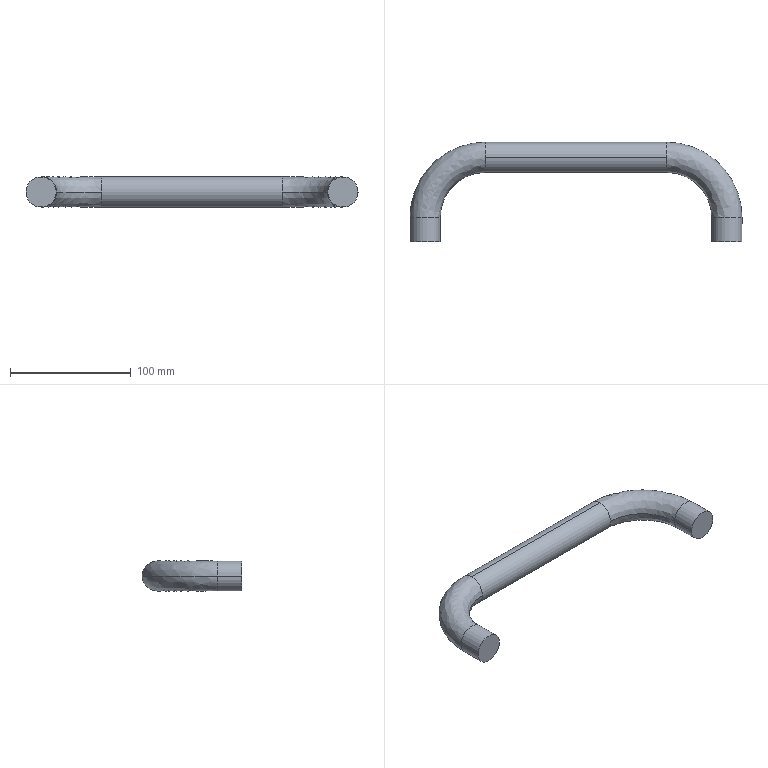Part | STEP file | 750078419 | 1 solid | 12 faces | box 275 x 82.5 x 25 mm | volume 170372 mm3 | cylinder 6 | spline 4 | plane 2 | commonest cylinder face diameters 25 x6
STEP:
#1=CARTESIAN_POINT('',(200.,82.5,0.));
#2=VERTEX_POINT('',#1);
#3=CARTESIAN_POINT('',(200.,70.,-12.5));
#4=VERTEX_POINT('',#3);
#5=CARTESIAN_POINT('',(200.,70.,0.));
#6=DIRECTION('',(-1.,0.,0.));
#7=DIRECTION('',(0.,0.,1.));
#8=AXIS2_PLACEMENT_3D('',#5,#6,#7);
#9=CIRCLE('',#8,12.5);
#10=EDGE_CURVE('',#2,#4,#9,.T.);
#11=ORIENTED_EDGE('',*,*,#10,.T.);
#12=CARTESIAN_POINT('',(50.,70.,-12.5));
#13=VERTEX_POINT('',#12);
#14=CARTESIAN_POINT('',(200.,70.,-12.5));
#15=DIRECTION('',(-1.,0.,0.));
#16=VECTOR('',#15,1000.);
#17=LINE('',#14,#16);
#18=EDGE_CURVE('',#4,#13,#17,.T.);
#19=ORIENTED_EDGE('',*,*,#18,.T.);
#20=CARTESIAN_POINT('',(50.,82.5,0.));
#21=VERTEX_POINT('',#20);
#22=CARTESIAN_POINT('',(50.,70.,0.));
#23=DIRECTION('',(1.,0.,0.));
#24=DIRECTION('',(0.,0.,1.));
#25=AXIS2_PLACEMENT_3D('',#22,#23,#24);
#26=CIRCLE('',#25,12.5);
#27=EDGE_CURVE('',#13,#21,#26,.T.);
#28=ORIENTED_EDGE('',*,*,#27,.T.);
#29=CARTESIAN_POINT('',(50.,70.,12.5));
#30=VERTEX_POINT('',#29);
#31=CARTESIAN_POINT('',(50.,70.,0.));
#32=DIRECTION('',(1.,0.,0.));
#33=DIRECTION('',(0.,0.,1.));
#34=AXIS2_PLACEMENT_3D('',#31,#32,#33);
#35=CIRCLE('',#34,12.5);
#36=EDGE_CURVE('',#21,#30,#35,.T.);
#37=ORIENTED_EDGE('',*,*,#36,.T.);
#38=CARTESIAN_POINT('',(200.,70.,12.5));
#39=VERTEX_POINT('',#38);
#40=CARTESIAN_POINT('',(200.,70.,12.5));
#41=DIRECTION('',(-1.,0.,0.));
#42=VECTOR('',#41,1000.);
#43=LINE('',#40,#42);
#44=EDGE_CURVE('',#39,#30,#43,.T.);
#45=ORIENTED_EDGE('',*,*,#44,.F.);
#46=CARTESIAN_POINT('',(200.,70.,0.));
#47=DIRECTION('',(-1.,0.,0.));
#48=DIRECTION('',(0.,0.,1.));
#49=AXIS2_PLACEMENT_3D('',#46,#47,#48);
#50=CIRCLE('',#49,12.5);
#51=EDGE_CURVE('',#39,#2,#50,.T.);
#52=ORIENTED_EDGE('',*,*,#51,.T.);
#53=EDGE_LOOP('',(#11,#19,#28,#37,#45,#52));
#54=FACE_OUTER_BOUND('',#53,.T.);
#55=CARTESIAN_POINT('',(200.,70.,0.));
#56=DIRECTION('',(-1.,0.,0.));
#57=DIRECTION('',(0.,0.,1.));
#58=AXIS2_PLACEMENT_3D('',#55,#56,#57);
#59=CYLINDRICAL_SURFACE('',#58,12.5);
#60=ADVANCED_FACE('',(#54),#59,.T.);
#61=CARTESIAN_POINT('',(50.,57.5,0.));
#62=VERTEX_POINT('',#61);
#63=CARTESIAN_POINT('',(50.,70.,0.));
#64=DIRECTION('',(1.,0.,0.));
#65=DIRECTION('',(0.,0.,1.));
#66=AXIS2_PLACEMENT_3D('',#63,#64,#65);
#67=CIRCLE('',#66,12.5);
#68=EDGE_CURVE('',#62,#13,#67,.T.);
#69=ORIENTED_EDGE('',*,*,#68,.F.);
#70=CARTESIAN_POINT('',(12.5,20.,0.));
#71=VERTEX_POINT('',#70);
#72=CARTESIAN_POINT('',(50.,20.,0.));
#73=DIRECTION('',(0.,0.,1.));
#74=DIRECTION('',(1.,0.,0.));
#75=AXIS2_PLACEMENT_3D('',#72,#73,#74);
#76=CIRCLE('',#75,37.5);
#77=EDGE_CURVE('',#62,#71,#76,.T.);
#78=ORIENTED_EDGE('',*,*,#77,.T.);
#79=CARTESIAN_POINT('',(-12.5,20.,0.));
#80=VERTEX_POINT('',#79);
#81=CARTESIAN_POINT('',(0.,20.,0.));
#82=DIRECTION('',(0.,1.,0.));
#83=DIRECTION('',(-1.,0.,0.));
#84=AXIS2_PLACEMENT_3D('',#81,#82,#83);
#85=CIRCLE('',#84,12.5);
#86=EDGE_CURVE('',#71,#80,#85,.T.);
#87=ORIENTED_EDGE('',*,*,#86,.T.);
#88=CARTESIAN_POINT('',(50.,20.,0.));
#89=DIRECTION('',(0.,0.,1.));
#90=DIRECTION('',(1.,0.,0.));
#91=AXIS2_PLACEMENT_3D('',#88,#89,#90);
#92=CIRCLE('',#91,62.5);
#93=EDGE_CURVE('',#21,#80,#92,.T.);
#94=ORIENTED_EDGE('',*,*,#93,.F.);
#95=ORIENTED_EDGE('',*,*,#27,.F.);
#96=EDGE_LOOP('',(#69,#78,#87,#94,#95));
#97=FACE_OUTER_BOUND('',#96,.T.);
#98=CARTESIAN_POINT('',(50.,82.5,0.));
#99=CARTESIAN_POINT('',(13.388,82.5,0.));
#100=CARTESIAN_POINT('',(-12.5,56.612,0.));
#101=CARTESIAN_POINT('',(-12.5,20.,0.));
#102=CARTESIAN_POINT('',(50.,82.5,-25.));
#103=CARTESIAN_POINT('',(13.388,82.5,-25.));
#104=CARTESIAN_POINT('',(-12.5,56.612,-25.));
#105=CARTESIAN_POINT('',(-12.5,20.,-25.));
#106=CARTESIAN_POINT('',(50.,57.5,-25.));
#107=CARTESIAN_POINT('',(28.033,57.5,-25.));
#108=CARTESIAN_POINT('',(12.5,41.967,-25.));
#109=CARTESIAN_POINT('',(12.5,20.,-25.));
#110=CARTESIAN_POINT('',(50.,57.5,0.));
#111=CARTESIAN_POINT('',(28.033,57.5,0.));
#112=CARTESIAN_POINT('',(12.5,41.967,0.));
#113=CARTESIAN_POINT('',(12.5,20.,0.));
#114=(BOUNDED_SURFACE()B_SPLINE_SURFACE(3,3,((#98,#99,#100,#101),(#102,#103,#104,#105),(#106,#107,#108,#109),(#110,#111,#112,#113)),.UNSPECIFIED.,.F.,.F.,.F.)B_SPLINE_SURFACE_WITH_KNOTS((4,4),(4,4),(0.,1.),(0.,1.),.UNSPECIFIED.)GEOMETRIC_REPRESENTATION_ITEM()RATIONAL_B_SPLINE_SURFACE(((1.,0.8047,0.8047,1.),(0.3333,0.2682,0.2682,0.3333),(0.3333,0.2682,0.2682,0.3333),(1.,0.8047,0.8047,1.)))REPRESENTATION_ITEM('')SURFACE());
#115=ADVANCED_FACE('',(#97),#114,.T.);
#116=CARTESIAN_POINT('',(262.5,20.,0.));
#117=VERTEX_POINT('',#116);
#118=CARTESIAN_POINT('',(237.5,20.,0.));
#119=VERTEX_POINT('',#118);
#120=CARTESIAN_POINT('',(250.,20.,0.));
#121=DIRECTION('',(0.,1.,0.));
#122=DIRECTION('',(1.,0.,0.));
#123=AXIS2_PLACEMENT_3D('',#120,#121,#122);
#124=CIRCLE('',#123,12.5);
#125=EDGE_CURVE('',#117,#119,#124,.T.);
#126=ORIENTED_EDGE('',*,*,#125,.T.);
#127=CARTESIAN_POINT('',(200.,57.5,0.));
#128=VERTEX_POINT('',#127);
#129=CARTESIAN_POINT('',(200.,20.,0.));
#130=DIRECTION('',(0.,0.,1.));
#131=DIRECTION('',(1.,0.,0.));
#132=AXIS2_PLACEMENT_3D('',#129,#130,#131);
#133=CIRCLE('',#132,37.5);
#134=EDGE_CURVE('',#119,#128,#133,.T.);
#135=ORIENTED_EDGE('',*,*,#134,.T.);
#136=CARTESIAN_POINT('',(200.,70.,0.));
#137=DIRECTION('',(-1.,0.,0.));
#138=DIRECTION('',(0.,0.,1.));
#139=AXIS2_PLACEMENT_3D('',#136,#137,#138);
#140=CIRCLE('',#139,12.5);
#141=EDGE_CURVE('',#4,#128,#140,.T.);
#142=ORIENTED_EDGE('',*,*,#141,.F.);
#143=ORIENTED_EDGE('',*,*,#10,.F.);
#144=CARTESIAN_POINT('',(200.,20.,0.));
#145=DIRECTION('',(0.,0.,1.));
#146=DIRECTION('',(1.,0.,0.));
#147=AXIS2_PLACEMENT_3D('',#144,#145,#146);
#148=CIRCLE('',#147,62.5);
#149=EDGE_CURVE('',#117,#2,#148,.T.);
#150=ORIENTED_EDGE('',*,*,#149,.F.);
#151=EDGE_LOOP('',(#126,#135,#142,#143,#150));
#152=FACE_OUTER_BOUND('',#151,.T.);
#153=CARTESIAN_POINT('',(262.5,20.,0.));
#154=CARTESIAN_POINT('',(262.5,56.612,0.));
#155=CARTESIAN_POINT('',(236.612,82.5,0.));
#156=CARTESIAN_POINT('',(200.,82.5,0.));
#157=CARTESIAN_POINT('',(262.5,20.,-25.));
#158=CARTESIAN_POINT('',(262.5,56.612,-25.));
#159=CARTESIAN_POINT('',(236.612,82.5,-25.));
#160=CARTESIAN_POINT('',(200.,82.5,-25.));
#161=CARTESIAN_POINT('',(237.5,20.,-25.));
#162=CARTESIAN_POINT('',(237.5,41.967,-25.));
#163=CARTESIAN_POINT('',(221.967,57.5,-25.));
#164=CARTESIAN_POINT('',(200.,57.5,-25.));
#165=CARTESIAN_POINT('',(237.5,20.,0.));
#166=CARTESIAN_POINT('',(237.5,41.967,0.));
#167=CARTESIAN_POINT('',(221.967,57.5,0.));
#168=CARTESIAN_POINT('',(200.,57.5,0.));
#169=(BOUNDED_SURFACE()B_SPLINE_SURFACE(3,3,((#153,#154,#155,#156),(#157,#158,#159,#160),(#161,#162,#163,#164),(#165,#166,#167,#168)),.UNSPECIFIED.,.F.,.F.,.T.)B_SPLINE_SURFACE_WITH_KNOTS((4,4),(4,4),(0.,1.),(0.,1.),.UNSPECIFIED.)GEOMETRIC_REPRESENTATION_ITEM()RATIONAL_B_SPLINE_SURFACE(((1.,0.8047,0.8047,1.),(0.3333,0.2682,0.2682,0.3333),(0.3333,0.2682,0.2682,0.3333),(1.,0.8047,0.8047,1.)))REPRESENTATION_ITEM('')SURFACE());
#170=ADVANCED_FACE('',(#152),#169,.T.);
#171=CARTESIAN_POINT('',(0.,20.,0.));
#172=DIRECTION('',(0.,1.,0.));
#173=DIRECTION('',(-1.,0.,0.));
#174=AXIS2_PLACEMENT_3D('',#171,#172,#173);
#175=CIRCLE('',#174,12.5);
#176=EDGE_CURVE('',#80,#71,#175,.T.);
#177=ORIENTED_EDGE('',*,*,#176,.F.);
#178=CARTESIAN_POINT('',(-12.5,0.,0.));
#179=VERTEX_POINT('',#178);
#180=CARTESIAN_POINT('',(-12.5,20.,0.));
#181=DIRECTION('',(0.,-1.,0.));
#182=VECTOR('',#181,1000.);
#183=LINE('',#180,#182);
#184=EDGE_CURVE('',#80,#179,#183,.T.);
#185=ORIENTED_EDGE('',*,*,#184,.T.);
#186=CARTESIAN_POINT('',(12.5,0.,0.));
#187=VERTEX_POINT('',#186);
#188=CARTESIAN_POINT('',(0.,0.,0.));
#189=DIRECTION('',(0.,1.,0.));
#190=DIRECTION('',(1.,0.,0.));
#191=AXIS2_PLACEMENT_3D('',#188,#189,#190);
#192=CIRCLE('',#191,12.5);
#193=EDGE_CURVE('',#179,#187,#192,.T.);
#194=ORIENTED_EDGE('',*,*,#193,.T.);
#195=CARTESIAN_POINT('',(12.5,20.,0.));
#196=DIRECTION('',(0.,-1.,0.));
#197=VECTOR('',#196,1000.);
#198=LINE('',#195,#197);
#199=EDGE_CURVE('',#71,#187,#198,.T.);
#200=ORIENTED_EDGE('',*,*,#199,.F.);
#201=EDGE_LOOP('',(#177,#185,#194,#200));
#202=FACE_OUTER_BOUND('',#201,.T.);
#203=CARTESIAN_POINT('',(0.,20.,0.));
#204=DIRECTION('',(0.,-1.,0.));
#205=DIRECTION('',(1.,0.,0.));
#206=AXIS2_PLACEMENT_3D('',#203,#204,#205);
#207=CYLINDRICAL_SURFACE('',#206,12.5);
#208=ADVANCED_FACE('',(#202),#207,.T.);
#209=CARTESIAN_POINT('',(250.,20.,0.));
#210=DIRECTION('',(0.,1.,0.));
#211=DIRECTION('',(1.,0.,0.));
#212=AXIS2_PLACEMENT_3D('',#209,#210,#211);
#213=CIRCLE('',#212,12.5);
#214=EDGE_CURVE('',#119,#117,#213,.T.);
#215=ORIENTED_EDGE('',*,*,#214,.F.);
#216=CARTESIAN_POINT('',(237.5,0.,0.));
#217=VERTEX_POINT('',#216);
#218=CARTESIAN_POINT('',(237.5,20.,0.));
#219=DIRECTION('',(0.,-1.,0.));
#220=VECTOR('',#219,1000.);
#221=LINE('',#218,#220);
#222=EDGE_CURVE('',#119,#217,#221,.T.);
#223=ORIENTED_EDGE('',*,*,#222,.T.);
#224=CARTESIAN_POINT('',(262.5,0.,0.));
#225=VERTEX_POINT('',#224);
#226=CARTESIAN_POINT('',(250.,0.,0.));
#227=DIRECTION('',(0.,1.,0.));
#228=DIRECTION('',(1.,0.,0.));
#229=AXIS2_PLACEMENT_3D('',#226,#227,#228);
#230=CIRCLE('',#229,12.5);
#231=EDGE_CURVE('',#217,#225,#230,.T.);
#232=ORIENTED_EDGE('',*,*,#231,.T.);
#233=CARTESIAN_POINT('',(262.5,20.,0.));
#234=DIRECTION('',(0.,-1.,0.));
#235=VECTOR('',#234,1000.);
#236=LINE('',#233,#235);
#237=EDGE_CURVE('',#117,#225,#236,.T.);
#238=ORIENTED_EDGE('',*,*,#237,.F.);
#239=EDGE_LOOP('',(#215,#223,#232,#238));
#240=FACE_OUTER_BOUND('',#239,.T.);
#241=CARTESIAN_POINT('',(250.,20.,0.));
#242=DIRECTION('',(0.,-1.,0.));
#243=DIRECTION('',(1.,0.,0.));
#244=AXIS2_PLACEMENT_3D('',#241,#242,#243);
#245=CYLINDRICAL_SURFACE('',#244,12.5);
#246=ADVANCED_FACE('',(#240),#245,.T.);
#247=ORIENTED_EDGE('',*,*,#18,.F.);
#248=ORIENTED_EDGE('',*,*,#141,.T.);
#249=CARTESIAN_POINT('',(200.,70.,0.));
#250=DIRECTION('',(-1.,0.,0.));
#251=DIRECTION('',(0.,0.,1.));
#252=AXIS2_PLACEMENT_3D('',#249,#250,#251);
#253=CIRCLE('',#252,12.5);
#254=EDGE_CURVE('',#128,#39,#253,.T.);
#255=ORIENTED_EDGE('',*,*,#254,.T.);
#256=ORIENTED_EDGE('',*,*,#44,.T.);
#257=CARTESIAN_POINT('',(50.,70.,0.));
#258=DIRECTION('',(1.,0.,0.));
#259=DIRECTION('',(0.,0.,1.));
#260=AXIS2_PLACEMENT_3D('',#257,#258,#259);
#261=CIRCLE('',#260,12.5);
#262=EDGE_CURVE('',#30,#62,#261,.T.);
#263=ORIENTED_EDGE('',*,*,#262,.T.);
#264=ORIENTED_EDGE('',*,*,#68,.T.);
#265=EDGE_LOOP('',(#247,#248,#255,#256,#263,#264));
#266=FACE_OUTER_BOUND('',#265,.T.);
#267=CARTESIAN_POINT('',(200.,70.,0.));
#268=DIRECTION('',(-1.,0.,0.));
#269=DIRECTION('',(0.,0.,1.));
#270=AXIS2_PLACEMENT_3D('',#267,#268,#269);
#271=CYLINDRICAL_SURFACE('',#270,12.5);
#272=ADVANCED_FACE('',(#266),#271,.T.);
#273=ORIENTED_EDGE('',*,*,#77,.F.);
#274=ORIENTED_EDGE('',*,*,#262,.F.);
#275=ORIENTED_EDGE('',*,*,#36,.F.);
#276=ORIENTED_EDGE('',*,*,#93,.T.);
#277=ORIENTED_EDGE('',*,*,#176,.T.);
#278=EDGE_LOOP('',(#273,#274,#275,#276,#277));
#279=FACE_OUTER_BOUND('',#278,.T.);
#280=CARTESIAN_POINT('',(50.,57.5,0.));
#281=CARTESIAN_POINT('',(28.033,57.5,0.));
#282=CARTESIAN_POINT('',(12.5,41.967,0.));
#283=CARTESIAN_POINT('',(12.5,20.,0.));
#284=CARTESIAN_POINT('',(50.,57.5,25.));
#285=CARTESIAN_POINT('',(28.033,57.5,25.));
#286=CARTESIAN_POINT('',(12.5,41.967,25.));
#287=CARTESIAN_POINT('',(12.5,20.,25.));
#288=CARTESIAN_POINT('',(50.,82.5,25.));
#289=CARTESIAN_POINT('',(13.388,82.5,25.));
#290=CARTESIAN_POINT('',(-12.5,56.612,25.));
#291=CARTESIAN_POINT('',(-12.5,20.,25.));
#292=CARTESIAN_POINT('',(50.,82.5,0.));
#293=CARTESIAN_POINT('',(13.388,82.5,0.));
#294=CARTESIAN_POINT('',(-12.5,56.612,0.));
#295=CARTESIAN_POINT('',(-12.5,20.,0.));
#296=(BOUNDED_SURFACE()B_SPLINE_SURFACE(3,3,((#280,#281,#282,#283),(#284,#285,#286,#287),(#288,#289,#290,#291),(#292,#293,#294,#295)),.UNSPECIFIED.,.F.,.F.,.F.)B_SPLINE_SURFACE_WITH_KNOTS((4,4),(4,4),(0.,1.),(0.,1.),.UNSPECIFIED.)GEOMETRIC_REPRESENTATION_ITEM()RATIONAL_B_SPLINE_SURFACE(((1.,0.8047,0.8047,1.),(0.3333,0.2682,0.2682,0.3333),(0.3333,0.2682,0.2682,0.3333),(1.,0.8047,0.8047,1.)))REPRESENTATION_ITEM('')SURFACE());
#297=ADVANCED_FACE('',(#279),#296,.T.);
#298=ORIENTED_EDGE('',*,*,#134,.F.);
#299=ORIENTED_EDGE('',*,*,#214,.T.);
#300=ORIENTED_EDGE('',*,*,#149,.T.);
#301=ORIENTED_EDGE('',*,*,#51,.F.);
#302=ORIENTED_EDGE('',*,*,#254,.F.);
#303=EDGE_LOOP('',(#298,#299,#300,#301,#302));
#304=FACE_OUTER_BOUND('',#303,.T.);
#305=CARTESIAN_POINT('',(237.5,20.,0.));
#306=CARTESIAN_POINT('',(237.5,41.967,0.));
#307=CARTESIAN_POINT('',(221.967,57.5,0.));
#308=CARTESIAN_POINT('',(200.,57.5,0.));
#309=CARTESIAN_POINT('',(237.5,20.,25.));
#310=CARTESIAN_POINT('',(237.5,41.967,25.));
#311=CARTESIAN_POINT('',(221.967,57.5,25.));
#312=CARTESIAN_POINT('',(200.,57.5,25.));
#313=CARTESIAN_POINT('',(262.5,20.,25.));
#314=CARTESIAN_POINT('',(262.5,56.612,25.));
#315=CARTESIAN_POINT('',(236.612,82.5,25.));
#316=CARTESIAN_POINT('',(200.,82.5,25.));
#317=CARTESIAN_POINT('',(262.5,20.,0.));
#318=CARTESIAN_POINT('',(262.5,56.612,0.));
#319=CARTESIAN_POINT('',(236.612,82.5,0.));
#320=CARTESIAN_POINT('',(200.,82.5,0.));
#321=(BOUNDED_SURFACE()B_SPLINE_SURFACE(3,3,((#305,#306,#307,#308),(#309,#310,#311,#312),(#313,#314,#315,#316),(#317,#318,#319,#320)),.UNSPECIFIED.,.F.,.F.,.F.)B_SPLINE_SURFACE_WITH_KNOTS((4,4),(4,4),(0.,1.),(0.,1.),.UNSPECIFIED.)GEOMETRIC_REPRESENTATION_ITEM()RATIONAL_B_SPLINE_SURFACE(((1.,0.8047,0.8047,1.),(0.3333,0.2682,0.2682,0.3333),(0.3333,0.2682,0.2682,0.3333),(1.,0.8047,0.8047,1.)))REPRESENTATION_ITEM('')SURFACE());
#322=ADVANCED_FACE('',(#304),#321,.T.);
#323=ORIENTED_EDGE('',*,*,#184,.F.);
#324=ORIENTED_EDGE('',*,*,#86,.F.);
#325=ORIENTED_EDGE('',*,*,#199,.T.);
#326=CARTESIAN_POINT('',(0.,0.,0.));
#327=DIRECTION('',(0.,1.,0.));
#328=DIRECTION('',(1.,0.,0.));
#329=AXIS2_PLACEMENT_3D('',#326,#327,#328);
#330=CIRCLE('',#329,12.5);
#331=EDGE_CURVE('',#187,#179,#330,.T.);
#332=ORIENTED_EDGE('',*,*,#331,.T.);
#333=EDGE_LOOP('',(#323,#324,#325,#332));
#334=FACE_OUTER_BOUND('',#333,.T.);
#335=CARTESIAN_POINT('',(0.,20.,0.));
#336=DIRECTION('',(0.,-1.,0.));
#337=DIRECTION('',(1.,0.,0.));
#338=AXIS2_PLACEMENT_3D('',#335,#336,#337);
#339=CYLINDRICAL_SURFACE('',#338,12.5);
#340=ADVANCED_FACE('',(#334),#339,.T.);
#341=ORIENTED_EDGE('',*,*,#222,.F.);
#342=ORIENTED_EDGE('',*,*,#125,.F.);
#343=ORIENTED_EDGE('',*,*,#237,.T.);
#344=CARTESIAN_POINT('',(250.,0.,0.));
#345=DIRECTION('',(0.,1.,0.));
#346=DIRECTION('',(1.,0.,0.));
#347=AXIS2_PLACEMENT_3D('',#344,#345,#346);
#348=CIRCLE('',#347,12.5);
#349=EDGE_CURVE('',#225,#217,#348,.T.);
#350=ORIENTED_EDGE('',*,*,#349,.T.);
#351=EDGE_LOOP('',(#341,#342,#343,#350));
#352=FACE_OUTER_BOUND('',#351,.T.);
#353=CARTESIAN_POINT('',(250.,20.,0.));
#354=DIRECTION('',(0.,-1.,0.));
#355=DIRECTION('',(1.,0.,0.));
#356=AXIS2_PLACEMENT_3D('',#353,#354,#355);
#357=CYLINDRICAL_SURFACE('',#356,12.5);
#358=ADVANCED_FACE('',(#352),#357,.T.);
#359=ORIENTED_EDGE('',*,*,#331,.F.);
#360=ORIENTED_EDGE('',*,*,#193,.F.);
#361=EDGE_LOOP('',(#359,#360));
#362=FACE_OUTER_BOUND('',#361,.T.);
#363=CARTESIAN_POINT('',(0.,0.,0.));
#364=DIRECTION('',(0.,-1.,0.));
#365=DIRECTION('',(1.,0.,0.));
#366=AXIS2_PLACEMENT_3D('',#363,#364,#365);
#367=PLANE('',#366);
#368=ADVANCED_FACE('',(#362),#367,.T.);
#369=ORIENTED_EDGE('',*,*,#349,.F.);
#370=ORIENTED_EDGE('',*,*,#231,.F.);
#371=EDGE_LOOP('',(#369,#370));
#372=FACE_OUTER_BOUND('',#371,.T.);
#373=CARTESIAN_POINT('',(250.,0.,0.));
#374=DIRECTION('',(0.,1.,0.));
#375=DIRECTION('',(-1.,0.,0.));
#376=AXIS2_PLACEMENT_3D('',#373,#374,#375);
#377=PLANE('',#376);
#378=ADVANCED_FACE('',(#372),#377,.F.);
#379=CLOSED_SHELL('',(#60,#115,#170,#208,#246,#272,#297,#322,#340,#358,#368,#378));
#380=MANIFOLD_SOLID_BREP('',#379);
#381=CARTESIAN_POINT('',(0.,0.,0.));
#382=DIRECTION('',(0.,0.,1.));
#383=DIRECTION('',(1.,0.,0.));
#384=AXIS2_PLACEMENT_3D('',#381,#382,#383);
#385=(LENGTH_UNIT()NAMED_UNIT(*)SI_UNIT(.MILLI.,.METRE.));
#386=UNCERTAINTY_MEASURE_WITH_UNIT(LENGTH_MEASURE(0.00001),#385,'','');
#387=(NAMED_UNIT(*)PLANE_ANGLE_UNIT()SI_UNIT($,.RADIAN.));
#388=(NAMED_UNIT(*)SI_UNIT($,.STERADIAN.)SOLID_ANGLE_UNIT());
#389=(GEOMETRIC_REPRESENTATION_CONTEXT(3)GLOBAL_UNCERTAINTY_ASSIGNED_CONTEXT((#386))GLOBAL_UNIT_ASSIGNED_CONTEXT((#385,#387,#388))REPRESENTATION_CONTEXT('',''));
#390=ADVANCED_BREP_SHAPE_REPRESENTATION('',(#380,#384),#389);